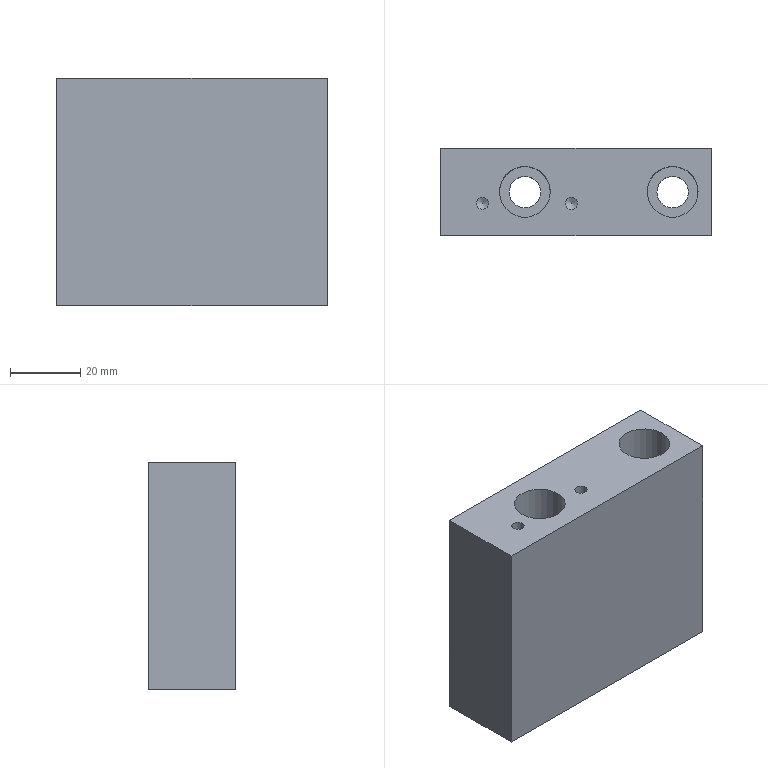Part | NX | features LB-4 2 | 1 solid | 16 faces | box 77.2 x 25 x 65 mm | volume 107840 mm3 | plane 8 | cylinder 6 | cone 2 | commonest cylinder face diameters 3.506 x2 9.007 x2 14.5 x2
STEP:
#1=CARTESIAN_POINT('',(2494.122,-1026.22,868.716));
#2=VERTEX_POINT('',#1);
#3=CARTESIAN_POINT('',(2492.369,-1026.22,868.716));
#4=DIRECTION('',(0.,0.,1.));
#5=DIRECTION('',(1.,0.,0.));
#6=AXIS2_PLACEMENT_3D('',#3,#4,#5);
#7=CIRCLE('',#6,1.753);
#8=EDGE_CURVE('',#2,#2,#7,.F.);
#9=ORIENTED_EDGE('',*,*,#8,.T.);
#10=EDGE_LOOP('',(#9));
#11=FACE_BOUND('',#10,.T.);
#12=CARTESIAN_POINT('',(2468.713,-1026.187,868.716));
#13=VERTEX_POINT('',#12);
#14=CARTESIAN_POINT('',(2466.96,-1026.187,868.716));
#15=DIRECTION('',(0.,0.,1.));
#16=DIRECTION('',(1.,0.,0.));
#17=AXIS2_PLACEMENT_3D('',#14,#15,#16);
#18=CIRCLE('',#17,1.753);
#19=EDGE_CURVE('',#13,#13,#18,.F.);
#20=ORIENTED_EDGE('',*,*,#19,.T.);
#21=EDGE_LOOP('',(#20));
#22=FACE_BOUND('',#21,.T.);
#23=CARTESIAN_POINT('',(2486.319,-1022.92,868.716));
#24=VERTEX_POINT('',#23);
#25=CARTESIAN_POINT('',(2479.069,-1022.92,868.716));
#26=DIRECTION('',(0.,0.,1.));
#27=DIRECTION('',(1.,0.,0.));
#28=AXIS2_PLACEMENT_3D('',#25,#26,#27);
#29=CIRCLE('',#28,7.25);
#30=EDGE_CURVE('',#24,#24,#29,.T.);
#31=ORIENTED_EDGE('',*,*,#30,.F.);
#32=EDGE_LOOP('',(#31));
#33=FACE_BOUND('',#32,.T.);
#34=CARTESIAN_POINT('',(2528.519,-1022.92,868.716));
#35=VERTEX_POINT('',#34);
#36=CARTESIAN_POINT('',(2521.269,-1022.92,868.716));
#37=DIRECTION('',(0.,0.,1.));
#38=DIRECTION('',(1.,0.,0.));
#39=AXIS2_PLACEMENT_3D('',#36,#37,#38);
#40=CIRCLE('',#39,7.25);
#41=EDGE_CURVE('',#35,#35,#40,.T.);
#42=ORIENTED_EDGE('',*,*,#41,.F.);
#43=EDGE_LOOP('',(#42));
#44=FACE_BOUND('',#43,.T.);
#45=CARTESIAN_POINT('',(2532.269,-1035.42,868.716));
#46=VERTEX_POINT('',#45);
#47=CARTESIAN_POINT('',(2455.069,-1035.42,868.716));
#48=VERTEX_POINT('',#47);
#49=CARTESIAN_POINT('',(2472.469,-1035.42,868.716));
#50=DIRECTION('',(-1.,0.,0.));
#51=VECTOR('',#50,1000.);
#52=LINE('',#49,#51);
#53=EDGE_CURVE('',#46,#48,#52,.T.);
#54=ORIENTED_EDGE('',*,*,#53,.F.);
#55=CARTESIAN_POINT('',(2532.269,-1010.42,868.716));
#56=VERTEX_POINT('',#55);
#57=CARTESIAN_POINT('',(2532.269,-1028.17,868.716));
#58=DIRECTION('',(0.,-1.,0.));
#59=VECTOR('',#58,1000.);
#60=LINE('',#57,#59);
#61=EDGE_CURVE('',#56,#46,#60,.T.);
#62=ORIENTED_EDGE('',*,*,#61,.F.);
#63=CARTESIAN_POINT('',(2455.069,-1010.42,868.716));
#64=VERTEX_POINT('',#63);
#65=CARTESIAN_POINT('',(2479.669,-1010.42,868.716));
#66=DIRECTION('',(1.,0.,0.));
#67=VECTOR('',#66,1000.);
#68=LINE('',#65,#67);
#69=EDGE_CURVE('',#64,#56,#68,.T.);
#70=ORIENTED_EDGE('',*,*,#69,.F.);
#71=CARTESIAN_POINT('',(2455.069,-1033.02,868.716));
#72=DIRECTION('',(0.,1.,0.));
#73=VECTOR('',#72,1000.);
#74=LINE('',#71,#73);
#75=EDGE_CURVE('',#48,#64,#74,.T.);
#76=ORIENTED_EDGE('',*,*,#75,.F.);
#77=EDGE_LOOP('',(#54,#62,#70,#76));
#78=FACE_BOUND('',#77,.T.);
#79=CARTESIAN_POINT('',(2450.149,-1036.87,868.716));
#80=DIRECTION('',(0.,0.,1.));
#81=DIRECTION('',(-1.,0.,0.));
#82=AXIS2_PLACEMENT_3D('',#79,#80,#81);
#83=PLANE('',#82);
#84=ADVANCED_FACE('',(#11,#22,#33,#44,#78),#83,.T.);
#85=CARTESIAN_POINT('',(2532.269,-1035.42,803.716));
#86=VERTEX_POINT('',#85);
#87=CARTESIAN_POINT('',(2532.269,-1035.42,876.911));
#88=DIRECTION('',(0.,0.,1.));
#89=VECTOR('',#88,1000.);
#90=LINE('',#87,#89);
#91=EDGE_CURVE('',#86,#46,#90,.T.);
#92=ORIENTED_EDGE('',*,*,#91,.T.);
#93=ORIENTED_EDGE('',*,*,#53,.T.);
#94=CARTESIAN_POINT('',(2455.069,-1035.42,803.716));
#95=VERTEX_POINT('',#94);
#96=CARTESIAN_POINT('',(2455.069,-1035.42,855.971));
#97=DIRECTION('',(0.,0.,1.));
#98=VECTOR('',#97,1000.);
#99=LINE('',#96,#98);
#100=EDGE_CURVE('',#95,#48,#99,.T.);
#101=ORIENTED_EDGE('',*,*,#100,.F.);
#102=CARTESIAN_POINT('',(2472.469,-1035.42,803.716));
#103=DIRECTION('',(1.,0.,0.));
#104=VECTOR('',#103,1000.);
#105=LINE('',#102,#104);
#106=EDGE_CURVE('',#95,#86,#105,.T.);
#107=ORIENTED_EDGE('',*,*,#106,.T.);
#108=EDGE_LOOP('',(#92,#93,#101,#107));
#109=FACE_BOUND('',#108,.T.);
#110=CARTESIAN_POINT('',(2472.469,-1035.42,876.911));
#111=DIRECTION('',(0.,-1.,0.));
#112=DIRECTION('',(0.,0.,1.));
#113=AXIS2_PLACEMENT_3D('',#110,#111,#112);
#114=PLANE('',#113);
#115=ADVANCED_FACE('',(#109),#114,.T.);
#116=ORIENTED_EDGE('',*,*,#100,.T.);
#117=ORIENTED_EDGE('',*,*,#75,.T.);
#118=CARTESIAN_POINT('',(2455.069,-1010.42,803.716));
#119=VERTEX_POINT('',#118);
#120=CARTESIAN_POINT('',(2455.069,-1010.42,803.716));
#121=DIRECTION('',(0.,0.,1.));
#122=VECTOR('',#121,1000.);
#123=LINE('',#120,#122);
#124=EDGE_CURVE('',#119,#64,#123,.T.);
#125=ORIENTED_EDGE('',*,*,#124,.F.);
#126=CARTESIAN_POINT('',(2455.069,-1033.02,803.716));
#127=DIRECTION('',(0.,-1.,0.));
#128=VECTOR('',#127,1000.);
#129=LINE('',#126,#128);
#130=EDGE_CURVE('',#119,#95,#129,.T.);
#131=ORIENTED_EDGE('',*,*,#130,.T.);
#132=EDGE_LOOP('',(#116,#117,#125,#131));
#133=FACE_BOUND('',#132,.T.);
#134=CARTESIAN_POINT('',(2455.069,-1033.02,855.971));
#135=DIRECTION('',(-1.,0.,0.));
#136=DIRECTION('',(0.,0.,-1.));
#137=AXIS2_PLACEMENT_3D('',#134,#135,#136);
#138=PLANE('',#137);
#139=ADVANCED_FACE('',(#133),#138,.T.);
#140=ORIENTED_EDGE('',*,*,#124,.T.);
#141=ORIENTED_EDGE('',*,*,#69,.T.);
#142=CARTESIAN_POINT('',(2532.269,-1010.42,803.716));
#143=VERTEX_POINT('',#142);
#144=CARTESIAN_POINT('',(2532.269,-1010.42,803.716));
#145=DIRECTION('',(0.,0.,1.));
#146=VECTOR('',#145,1000.);
#147=LINE('',#144,#146);
#148=EDGE_CURVE('',#143,#56,#147,.T.);
#149=ORIENTED_EDGE('',*,*,#148,.F.);
#150=CARTESIAN_POINT('',(2479.669,-1010.42,803.716));
#151=DIRECTION('',(-1.,0.,0.));
#152=VECTOR('',#151,1000.);
#153=LINE('',#150,#152);
#154=EDGE_CURVE('',#143,#119,#153,.T.);
#155=ORIENTED_EDGE('',*,*,#154,.T.);
#156=EDGE_LOOP('',(#140,#141,#149,#155));
#157=FACE_BOUND('',#156,.T.);
#158=CARTESIAN_POINT('',(2479.669,-1010.42,803.716));
#159=DIRECTION('',(0.,1.,0.));
#160=DIRECTION('',(0.,0.,-1.));
#161=AXIS2_PLACEMENT_3D('',#158,#159,#160);
#162=PLANE('',#161);
#163=ADVANCED_FACE('',(#157),#162,.T.);
#164=CARTESIAN_POINT('',(2474.565,-1022.92,803.716));
#165=VERTEX_POINT('',#164);
#166=CARTESIAN_POINT('',(2479.069,-1022.92,803.716));
#167=DIRECTION('',(0.,0.,-1.));
#168=DIRECTION('',(-1.,0.,0.));
#169=AXIS2_PLACEMENT_3D('',#166,#167,#168);
#170=CIRCLE('',#169,4.503);
#171=EDGE_CURVE('',#165,#165,#170,.F.);
#172=ORIENTED_EDGE('',*,*,#171,.T.);
#173=EDGE_LOOP('',(#172));
#174=FACE_BOUND('',#173,.T.);
#175=CARTESIAN_POINT('',(2516.765,-1022.92,803.716));
#176=VERTEX_POINT('',#175);
#177=CARTESIAN_POINT('',(2521.269,-1022.92,803.716));
#178=DIRECTION('',(0.,0.,-1.));
#179=DIRECTION('',(-1.,0.,0.));
#180=AXIS2_PLACEMENT_3D('',#177,#178,#179);
#181=CIRCLE('',#180,4.503);
#182=EDGE_CURVE('',#176,#176,#181,.F.);
#183=ORIENTED_EDGE('',*,*,#182,.T.);
#184=EDGE_LOOP('',(#183));
#185=FACE_BOUND('',#184,.T.);
#186=CARTESIAN_POINT('',(2532.269,-1028.17,803.716));
#187=DIRECTION('',(0.,1.,0.));
#188=VECTOR('',#187,1000.);
#189=LINE('',#186,#188);
#190=EDGE_CURVE('',#86,#143,#189,.T.);
#191=ORIENTED_EDGE('',*,*,#190,.F.);
#192=ORIENTED_EDGE('',*,*,#106,.F.);
#193=ORIENTED_EDGE('',*,*,#130,.F.);
#194=ORIENTED_EDGE('',*,*,#154,.F.);
#195=EDGE_LOOP('',(#191,#192,#193,#194));
#196=FACE_BOUND('',#195,.T.);
#197=CARTESIAN_POINT('',(2479.669,-1028.17,803.716));
#198=DIRECTION('',(0.,0.,-1.));
#199=DIRECTION('',(1.,0.,0.));
#200=AXIS2_PLACEMENT_3D('',#197,#198,#199);
#201=PLANE('',#200);
#202=ADVANCED_FACE('',(#174,#185,#196),#201,.T.);
#203=ORIENTED_EDGE('',*,*,#190,.T.);
#204=ORIENTED_EDGE('',*,*,#148,.T.);
#205=ORIENTED_EDGE('',*,*,#61,.T.);
#206=ORIENTED_EDGE('',*,*,#91,.F.);
#207=EDGE_LOOP('',(#203,#204,#205,#206));
#208=FACE_BOUND('',#207,.T.);
#209=CARTESIAN_POINT('',(2532.269,-1028.17,803.716));
#210=DIRECTION('',(1.,0.,0.));
#211=DIRECTION('',(0.,0.,1.));
#212=AXIS2_PLACEMENT_3D('',#209,#210,#211);
#213=PLANE('',#212);
#214=ADVANCED_FACE('',(#208),#213,.T.);
#215=CARTESIAN_POINT('',(2516.765,-1022.92,823.716));
#216=VERTEX_POINT('',#215);
#217=CARTESIAN_POINT('',(2521.269,-1022.92,823.716));
#218=DIRECTION('',(0.,0.,-1.));
#219=DIRECTION('',(-1.,0.,0.));
#220=AXIS2_PLACEMENT_3D('',#217,#218,#219);
#221=CIRCLE('',#220,4.503);
#222=EDGE_CURVE('',#216,#216,#221,.F.);
#223=ORIENTED_EDGE('',*,*,#222,.T.);
#224=EDGE_LOOP('',(#223));
#225=FACE_BOUND('',#224,.T.);
#226=ORIENTED_EDGE('',*,*,#182,.F.);
#227=EDGE_LOOP('',(#226));
#228=FACE_BOUND('',#227,.T.);
#229=CARTESIAN_POINT('',(2521.269,-1022.92,803.716));
#230=DIRECTION('',(0.,0.,1.));
#231=DIRECTION('',(-1.,0.,0.));
#232=AXIS2_PLACEMENT_3D('',#229,#230,#231);
#233=CYLINDRICAL_SURFACE('',#232,4.503);
#234=ADVANCED_FACE('',(#225,#228),#233,.F.);
#235=ORIENTED_EDGE('',*,*,#222,.F.);
#236=EDGE_LOOP('',(#235));
#237=FACE_BOUND('',#236,.T.);
#238=CARTESIAN_POINT('',(2514.019,-1022.92,823.716));
#239=VERTEX_POINT('',#238);
#240=CARTESIAN_POINT('',(2521.269,-1022.92,823.716));
#241=DIRECTION('',(0.,0.,-1.));
#242=DIRECTION('',(-1.,0.,0.));
#243=AXIS2_PLACEMENT_3D('',#240,#241,#242);
#244=CIRCLE('',#243,7.25);
#245=EDGE_CURVE('',#239,#239,#244,.T.);
#246=ORIENTED_EDGE('',*,*,#245,.F.);
#247=EDGE_LOOP('',(#246));
#248=FACE_BOUND('',#247,.T.);
#249=CARTESIAN_POINT('',(2521.269,-1022.92,823.716));
#250=DIRECTION('',(0.,0.,-1.));
#251=DIRECTION('',(1.,0.,0.));
#252=AXIS2_PLACEMENT_3D('',#249,#250,#251);
#253=PLANE('',#252);
#254=ADVANCED_FACE('',(#237,#248),#253,.F.);
#255=ORIENTED_EDGE('',*,*,#41,.T.);
#256=EDGE_LOOP('',(#255));
#257=FACE_BOUND('',#256,.T.);
#258=ORIENTED_EDGE('',*,*,#245,.T.);
#259=EDGE_LOOP('',(#258));
#260=FACE_BOUND('',#259,.T.);
#261=CARTESIAN_POINT('',(2521.269,-1022.92,823.716));
#262=DIRECTION('',(0.,0.,1.));
#263=DIRECTION('',(-1.,0.,0.));
#264=AXIS2_PLACEMENT_3D('',#261,#262,#263);
#265=CYLINDRICAL_SURFACE('',#264,7.25);
#266=ADVANCED_FACE('',(#257,#260),#265,.F.);
#267=CARTESIAN_POINT('',(2474.565,-1022.92,823.716));
#268=VERTEX_POINT('',#267);
#269=CARTESIAN_POINT('',(2479.069,-1022.92,823.716));
#270=DIRECTION('',(0.,0.,-1.));
#271=DIRECTION('',(-1.,0.,0.));
#272=AXIS2_PLACEMENT_3D('',#269,#270,#271);
#273=CIRCLE('',#272,4.503);
#274=EDGE_CURVE('',#268,#268,#273,.F.);
#275=ORIENTED_EDGE('',*,*,#274,.T.);
#276=EDGE_LOOP('',(#275));
#277=FACE_BOUND('',#276,.T.);
#278=ORIENTED_EDGE('',*,*,#171,.F.);
#279=EDGE_LOOP('',(#278));
#280=FACE_BOUND('',#279,.T.);
#281=CARTESIAN_POINT('',(2479.069,-1022.92,803.716));
#282=DIRECTION('',(0.,0.,1.));
#283=DIRECTION('',(-1.,0.,0.));
#284=AXIS2_PLACEMENT_3D('',#281,#282,#283);
#285=CYLINDRICAL_SURFACE('',#284,4.503);
#286=ADVANCED_FACE('',(#277,#280),#285,.F.);
#287=ORIENTED_EDGE('',*,*,#274,.F.);
#288=EDGE_LOOP('',(#287));
#289=FACE_BOUND('',#288,.T.);
#290=CARTESIAN_POINT('',(2471.819,-1022.92,823.716));
#291=VERTEX_POINT('',#290);
#292=CARTESIAN_POINT('',(2479.069,-1022.92,823.716));
#293=DIRECTION('',(0.,0.,-1.));
#294=DIRECTION('',(-1.,0.,0.));
#295=AXIS2_PLACEMENT_3D('',#292,#293,#294);
#296=CIRCLE('',#295,7.25);
#297=EDGE_CURVE('',#291,#291,#296,.T.);
#298=ORIENTED_EDGE('',*,*,#297,.F.);
#299=EDGE_LOOP('',(#298));
#300=FACE_BOUND('',#299,.T.);
#301=CARTESIAN_POINT('',(2479.069,-1022.92,823.716));
#302=DIRECTION('',(0.,0.,-1.));
#303=DIRECTION('',(1.,0.,0.));
#304=AXIS2_PLACEMENT_3D('',#301,#302,#303);
#305=PLANE('',#304);
#306=ADVANCED_FACE('',(#289,#300),#305,.F.);
#307=ORIENTED_EDGE('',*,*,#30,.T.);
#308=EDGE_LOOP('',(#307));
#309=FACE_BOUND('',#308,.T.);
#310=ORIENTED_EDGE('',*,*,#297,.T.);
#311=EDGE_LOOP('',(#310));
#312=FACE_BOUND('',#311,.T.);
#313=CARTESIAN_POINT('',(2479.069,-1022.92,823.716));
#314=DIRECTION('',(0.,0.,1.));
#315=DIRECTION('',(-1.,0.,0.));
#316=AXIS2_PLACEMENT_3D('',#313,#314,#315);
#317=CYLINDRICAL_SURFACE('',#316,7.25);
#318=ADVANCED_FACE('',(#309,#312),#317,.F.);
#319=CARTESIAN_POINT('',(2468.713,-1026.187,858.718));
#320=VERTEX_POINT('',#319);
#321=CARTESIAN_POINT('',(2466.96,-1026.187,858.718));
#322=DIRECTION('',(0.,0.,1.));
#323=DIRECTION('',(1.,0.,0.));
#324=AXIS2_PLACEMENT_3D('',#321,#322,#323);
#325=CIRCLE('',#324,1.753);
#326=EDGE_CURVE('',#320,#320,#325,.T.);
#327=ORIENTED_EDGE('',*,*,#326,.F.);
#328=EDGE_LOOP('',(#327));
#329=FACE_BOUND('',#328,.T.);
#330=ORIENTED_EDGE('',*,*,#19,.F.);
#331=EDGE_LOOP('',(#330));
#332=FACE_BOUND('',#331,.T.);
#333=CARTESIAN_POINT('',(2466.96,-1026.187,868.716));
#334=DIRECTION('',(0.,0.,-1.));
#335=DIRECTION('',(-1.,0.,0.));
#336=AXIS2_PLACEMENT_3D('',#333,#334,#335);
#337=CYLINDRICAL_SURFACE('',#336,1.753);
#338=ADVANCED_FACE('',(#329,#332),#337,.F.);
#339=ORIENTED_EDGE('',*,*,#326,.T.);
#340=EDGE_LOOP('',(#339));
#341=FACE_BOUND('',#340,.T.);
#342=CARTESIAN_POINT('',(2466.96,-1026.187,857.706));
#343=VERTEX_POINT('',#342);
#344=VERTEX_LOOP('',#343);
#345=FACE_BOUND('',#344,.T.);
#346=CARTESIAN_POINT('',(2466.96,-1026.187,857.706));
#347=DIRECTION('',(0.,0.,1.));
#348=DIRECTION('',(-1.,0.,0.));
#349=AXIS2_PLACEMENT_3D('',#346,#347,#348);
#350=CONICAL_SURFACE('',#349,0.,1.047);
#351=ADVANCED_FACE('',(#341,#345),#350,.F.);
#352=CARTESIAN_POINT('',(2494.122,-1026.22,858.718));
#353=VERTEX_POINT('',#352);
#354=CARTESIAN_POINT('',(2492.369,-1026.22,858.718));
#355=DIRECTION('',(0.,0.,1.));
#356=DIRECTION('',(1.,0.,0.));
#357=AXIS2_PLACEMENT_3D('',#354,#355,#356);
#358=CIRCLE('',#357,1.753);
#359=EDGE_CURVE('',#353,#353,#358,.T.);
#360=ORIENTED_EDGE('',*,*,#359,.F.);
#361=EDGE_LOOP('',(#360));
#362=FACE_BOUND('',#361,.T.);
#363=ORIENTED_EDGE('',*,*,#8,.F.);
#364=EDGE_LOOP('',(#363));
#365=FACE_BOUND('',#364,.T.);
#366=CARTESIAN_POINT('',(2492.369,-1026.22,868.716));
#367=DIRECTION('',(0.,0.,-1.));
#368=DIRECTION('',(-1.,0.,0.));
#369=AXIS2_PLACEMENT_3D('',#366,#367,#368);
#370=CYLINDRICAL_SURFACE('',#369,1.753);
#371=ADVANCED_FACE('',(#362,#365),#370,.F.);
#372=ORIENTED_EDGE('',*,*,#359,.T.);
#373=EDGE_LOOP('',(#372));
#374=FACE_BOUND('',#373,.T.);
#375=CARTESIAN_POINT('',(2492.369,-1026.22,857.706));
#376=VERTEX_POINT('',#375);
#377=VERTEX_LOOP('',#376);
#378=FACE_BOUND('',#377,.T.);
#379=CARTESIAN_POINT('',(2492.369,-1026.22,857.706));
#380=DIRECTION('',(0.,0.,1.));
#381=DIRECTION('',(-1.,0.,0.));
#382=AXIS2_PLACEMENT_3D('',#379,#380,#381);
#383=CONICAL_SURFACE('',#382,0.,1.047);
#384=ADVANCED_FACE('',(#374,#378),#383,.F.);
#385=CLOSED_SHELL('',(#84,#115,#139,#163,#202,#214,#234,#254,#266,#286,#306,#318,#338,#351,#371,#384));
#386=MANIFOLD_SOLID_BREP('',#385);
#387=(LENGTH_UNIT()NAMED_UNIT(*)SI_UNIT(.MILLI.,.METRE.));
#388=UNCERTAINTY_MEASURE_WITH_UNIT(LENGTH_MEASURE(0.00001),#387,'','');
#389=(NAMED_UNIT(*)PLANE_ANGLE_UNIT()SI_UNIT($,.RADIAN.));
#390=(NAMED_UNIT(*)SI_UNIT($,.STERADIAN.)SOLID_ANGLE_UNIT());
#391=(GEOMETRIC_REPRESENTATION_CONTEXT(3)GLOBAL_UNCERTAINTY_ASSIGNED_CONTEXT((#388))GLOBAL_UNIT_ASSIGNED_CONTEXT((#387,#389,#390))REPRESENTATION_CONTEXT('',''));
#392=ADVANCED_BREP_SHAPE_REPRESENTATION('',(#386),#391);